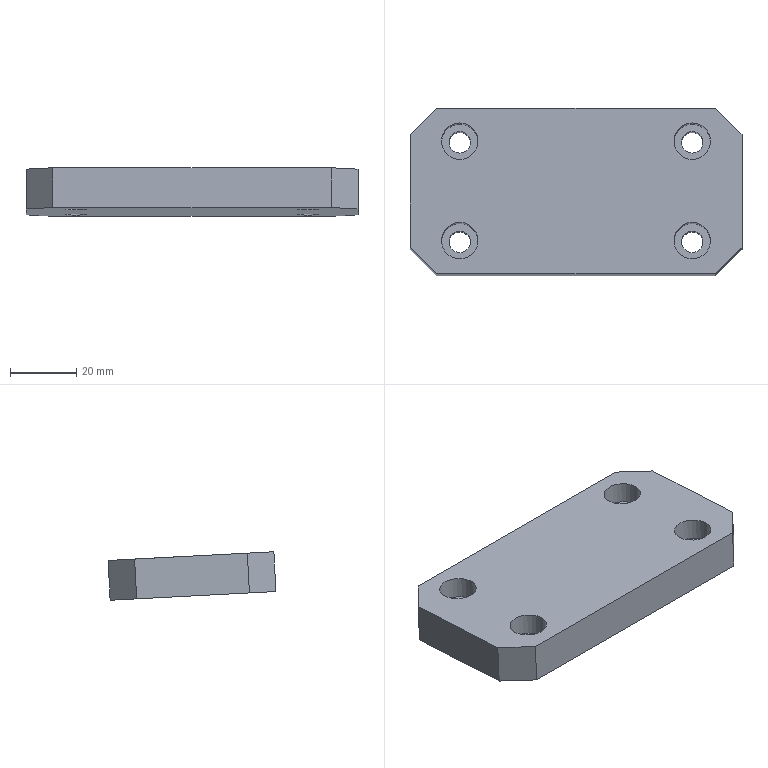Part | STEP file | P011002S001-006 | 1 solid | 22 faces | box 100 x 50.56 x 14.6 mm | volume 55263 mm3 | plane 14 | cylinder 8 | commonest cylinder face diameters 6.5 x4 11 x4